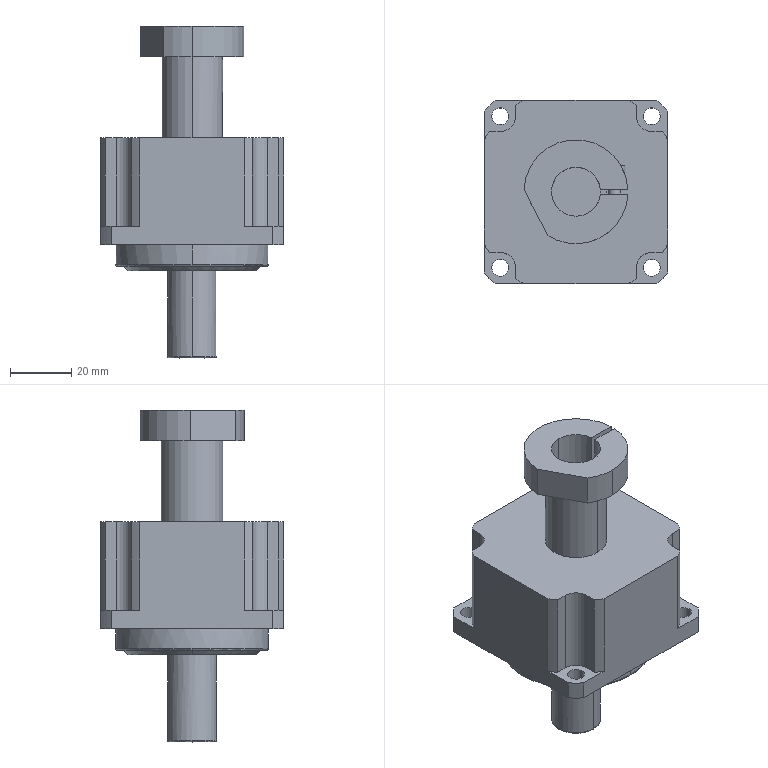Part | NX | 1 solid | 86 faces | box 60 x 60 x 108.5 mm | volume 146131 mm3 | cylinder 44 | plane 30 | cone 6 | torus 6 | commonest cylinder face diameters 5.5 x8 69 x8 10 x4 16 x4 80 x4 34 x3